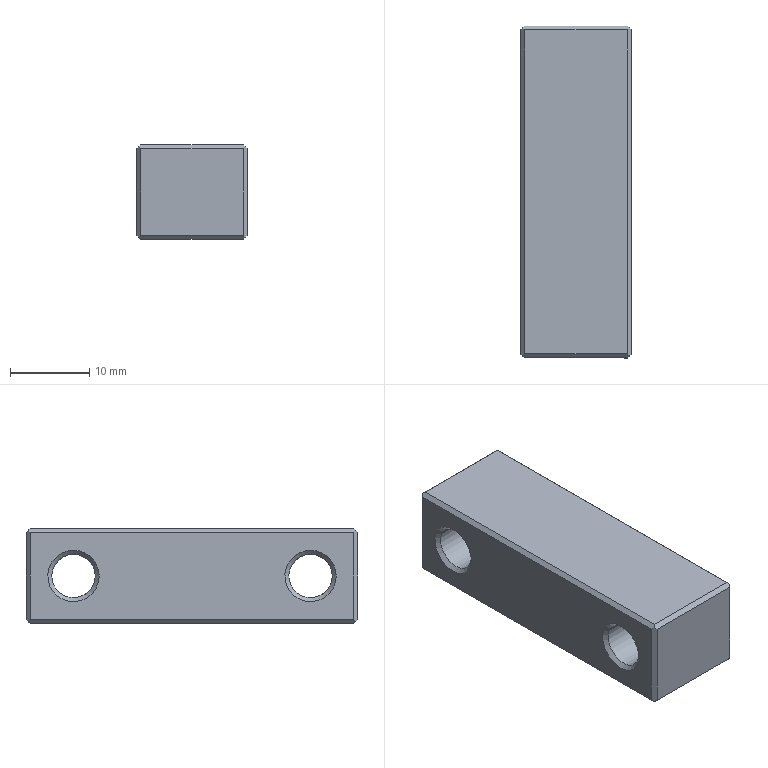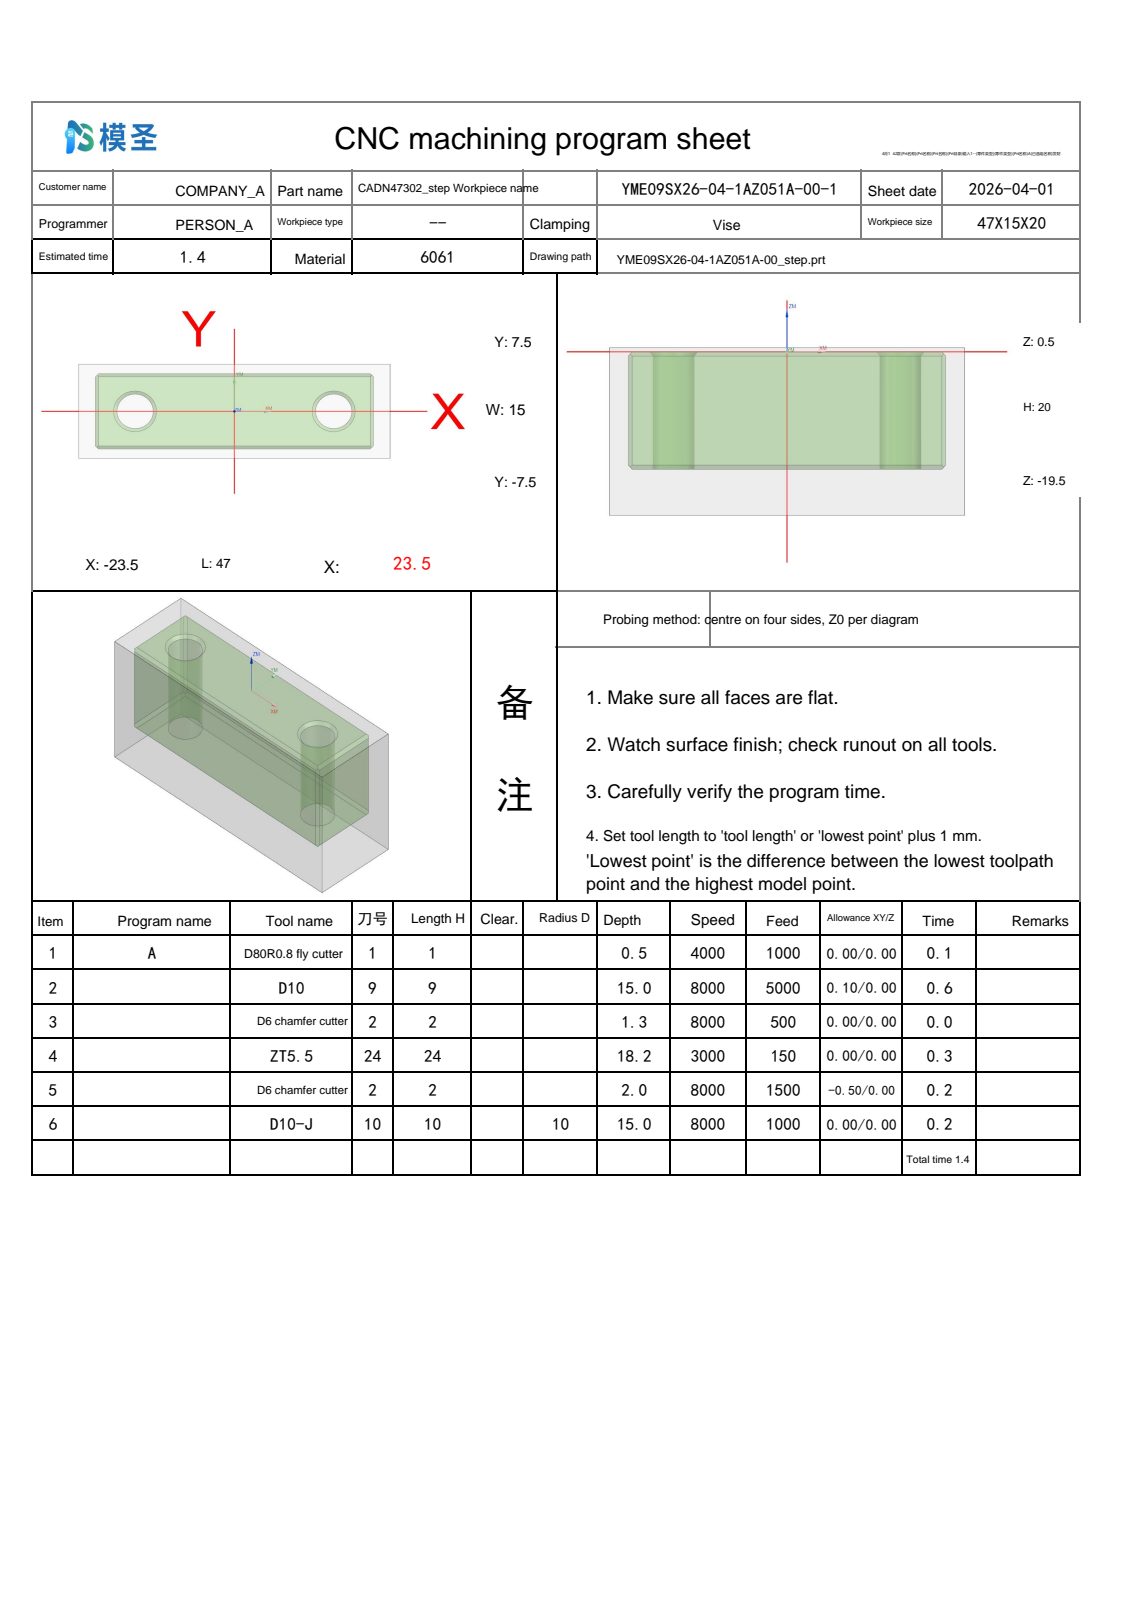NC program | NX | posted by the shop | part box 14 x 42 x 12 mm
Whole program:
%
O0001
(Machine time: 2.49 MIN)
(===Total Tool:5===)
(T1=D80R0.8 fly cutter D=80.  R=0.8  D-  H01 Z=0.    )
(T9=D10     D=10.  R=0.   D-  H09 Z=-14.5 )
(T2=D6 chamfer cutter   D=6.   R=0.   D-  H02 Z=-1.5  )
(T24=ZT5.5  D=5.5  DR_a=118 D-  H24 Z=-17.65)
(T10=D10-J  D=10.  R=0.   D10 H10 Z=-14.5 )
G80 G90 G17 G49 G40
G91 G28 Z0
M01
N1 T01 M06
(D80R0.8 fly cutter  D=80. R=0.8 H=01 ce=0.00 di=0.00)
G00 G90 G54 X-66. Y0.0 M03 S4000
G43 H01 Z20.
M08
Z2.
G01 Z0.0 F1000.
X-61.
X61.
X66.
Z2.
G00 Z20.
G91 G28 Z0.0
M05
M09
G91 G28 Z0.0
M01
N2 T09 M06
(D10  D=10. R=0. H=09 ce=0.10 di=0.00)
G00 G90 G54 X0.0 Y11.1 M03 S8000
G43 H09 Z20.
M08
Z.5
G01 X20.5 Z.383 F5000.
G02 X24.106 Y9.606 Z.361 I0.0 J-5.1
G01 X24.606 Y9.106 Z.357
G02 X26.1 Y5.5 Z.334 I-3.606 J-3.606
G01 Y-5.5 Z.271
G02 X24.606 Y-9.106 Z.249 I-5.1 J0.0
G01 X24.106 Y-9.606 Z.245
G02 X20.5 Y-11.1 Z.222 I-3.606 J3.606
G01 X-20.5 Z-.011
G02 X-24.106 Y-9.606 Z-.034 I0.0 J5.1
G01 X-24.606 Y-9.106 Z-.038
G02 X-26.1 Y-5.5 Z-.061 I3.606 J3.606
G01 Y5.5 Z-.123
G02 X-24.606 Y9.106 Z-.146 I5.1 J0.0
G01 X-24.106 Y9.606 Z-.15
G02 X-20.5 Y11.1 Z-.173 I3.606 J-3.606
G01 X20.5 Z-.406
G02 X24.106 Y9.606 Z-.429 I0.0 J-5.1
G01 X24.606 Y9.106 Z-.433
G02 X26.1 Y5.5 Z-.456 I-3.606 J-3.606
G01 Y-5.5 Z-.518
G02 X24.606 Y-9.106 Z-.541 I-5.1 J0.0
G01 X24.106 Y-9.606 Z-.545
G02 X20.5 Y-11.1 Z-.568 I-3.606 J3.606
G01 X-20.5 Z-.801
G02 X-24.106 Y-9.606 Z-.824 I0.0 J5.1
G01 X-24.606 Y-9.106 Z-.828
G02 X-26.1 Y-5.5 Z-.85 I3.606 J3.606
G01 Y5.5 Z-.913
G02 X-24.606 Y9.106 Z-.936 I5.1 J0.0
G01 X-24.106 Y9.606 Z-.94
G02 X-20.5 Y11.1 Z-.962 I3.606 J-3.606
G01 X20.5 Z-1.195
G02 X24.106 Y9.606 Z-1.218 I0.0 J-5.1
G01 X24.606 Y9.106 Z-1.222
G02 X26.1 Y5.5 Z-1.245 I-3.606 J-3.606
G01 Y-5.5 Z-1.308
G02 X24.606 Y-9.106 Z-1.33 I-5.1 J0.0
G01 X24.106 Y-9.606 Z-1.334
G02 X20.5 Y-11.1 Z-1.357 I-3.606 J3.606
G01 X-20.5 Z-1.59
G02 X-24.106 Y-9.606 Z-1.613 I0.0 J5.1
G01 X-24.606 Y-9.106 Z-1.617
G02 X-26.1 Y-5.5 Z-1.64 I3.606 J3.606
G01 Y5.5 Z-1.702
G02 X-24.606 Y9.106 Z-1.725 I5.1 J0.0
G01 X-24.106 Y9.606 Z-1.729
G02 X-20.5 Y11.1 Z-1.752 I3.606 J-3.606
G01 X20.5 Z-1.985
G02 X24.106 Y9.606 Z-2.008 I0.0 J-5.1
G01 X24.606 Y9.106 Z-2.012
G02 X26.1 Y5.5 Z-2.035 I-3.606 J-3.606
G01 Y-5.5 Z-2.097
G02 X24.606 Y-9.106 Z-2.12 I-5.1 J0.0
G01 X24.106 Y-9.606 Z-2.124
G02 X20.5 Y-11.1 Z-2.147 I-3.606 J3.606
G01 X-20.5 Z-2.38
G02 X-24.106 Y-9.606 Z-2.402 I0.0 J5.1
G01 X-24.606 Y-9.106 Z-2.406
G02 X-26.1 Y-5.5 Z-2.429 I3.606 J3.606
G01 Y5.5 Z-2.492
G02 X-24.606 Y9.106 Z-2.515 I5.1 J0.0
G01 X-24.106 Y9.606 Z-2.519
G02 X-20.5 Y11.1 Z-2.541 I3.606 J-3.606
G01 X20.5 Z-2.774
G02 X24.106 Y9.606 Z-2.797 I0.0 J-5.1
G01 X24.606 Y9.106 Z-2.801
G02 X26.1 Y5.5 Z-2.824 I-3.606 J-3.606
G01 Y-5.5 Z-2.887
G02 X24.606 Y-9.106 Z-2.909 I-5.1 J0.0
G01 X24.106 Y-9.606 Z-2.913
G02 X20.5 Y-11.1 Z-2.936 I-3.606 J3.606
G01 X-20.5 Z-3.169
G02 X-24.106 Y-9.606 Z-3.192 I0.0 J5.1
G01 X-24.606 Y-9.106 Z-3.196
G02 X-26.1 Y-5.5 Z-3.219 I3.606 J3.606
G01 Y5.5 Z-3.281
G02 X-24.606 Y9.106 Z-3.304 I5.1 J0.0
G01 X-24.106 Y9.606 Z-3.308
G02 X-20.5 Y11.1 Z-3.331 I3.606 J-3.606
G01 X20.5 Z-3.564
G02 X24.106 Y9.606 Z-3.587 I0.0 J-5.1
G01 X24.606 Y9.106 Z-3.591
G02 X26.1 Y5.5 Z-3.613 I-3.606 J-3.606
G01 Y-5.5 Z-3.676
G02 X24.606 Y-9.106 Z-3.699 I-5.1 J0.0
G01 X24.106 Y-9.606 Z-3.703
G02 X20.5 Y-11.1 Z-3.726 I-3.606 J3.606
G01 X-20.5 Z-3.959
G02 X-24.106 Y-9.606 Z-3.981 I0.0 J5.1
G01 X-24.606 Y-9.106 Z-3.985
G02 X-26.1 Y-5.5 Z-4.008 I3.606 J3.606
G01 Y5.5 Z-4.071
G02 X-24.606 Y9.106 Z-4.094 I5.1 J0.0
G01 X-24.106 Y9.606 Z-4.098
G02 X-20.5 Y11.1 Z-4.12 I3.606 J-3.606
G01 X20.5 Z-4.353
G02 X24.106 Y9.606 Z-4.376 I0.0 J-5.1
G01 X24.606 Y9.106 Z-4.38
G02 X26.1 Y5.5 Z-4.403 I-3.606 J-3.606
G01 Y-5.5 Z-4.465
G02 X24.606 Y-9.106 Z-4.488 I-5.1 J0.0
G01 X24.106 Y-9.606 Z-4.492
G02 X20.5 Y-11.1 Z-4.515 I-3.606 J3.606
G01 X-20.5 Z-4.748
G02 X-24.106 Y-9.606 Z-4.771 I0.0 J5.1
G01 X-24.606 Y-9.106 Z-4.775
G02 X-26.1 Y-5.5 Z-4.798 I3.606 J3.606
G01 Y5.5 Z-4.86
G02 X-24.606 Y9.106 Z-4.883 I5.1 J0.0
G01 X-24.106 Y9.606 Z-4.887
G02 X-20.5 Y11.1 Z-4.91 I3.606 J-3.606
G01 X20.5 Z-5.143
G02 X24.106 Y9.606 Z-5.166 I0.0 J-5.1
G01 X24.606 Y9.106 Z-5.17
G02 X26.1 Y5.5 Z-5.192 I-3.606 J-3.606
G01 Y-5.5 Z-5.255
G02 X24.606 Y-9.106 Z-5.278 I-5.1 J0.0
G01 X24.106 Y-9.606 Z-5.282
G02 X20.5 Y-11.1 Z-5.305 I-3.606 J3.606
G01 X-20.5 Z-5.538
G02 X-24.106 Y-9.606 Z-5.56 I0.0 J5.1
G01 X-24.606 Y-9.106 Z-5.564
G02 X-26.1 Y-5.5 Z-5.587 I3.606 J3.606
G01 Y5.5 Z-5.65
G02 X-24.606 Y9.106 Z-5.672 I5.1 J0.0
G01 X-24.106 Y9.606 Z-5.676
G02 X-20.5 Y11.1 Z-5.699 I3.606 J-3.606
G01 X20.5 Z-5.932
G02 X24.106 Y9.606 Z-5.955 I0.0 J-5.1
G01 X24.606 Y9.106 Z-5.959
G02 X26.1 Y5.5 Z-5.982 I-3.606 J-3.606
G01 Y-5.5 Z-6.044
G02 X24.606 Y-9.106 Z-6.067 I-5.1 J0.0
G01 X24.106 Y-9.606 Z-6.071
G02 X20.5 Y-11.1 Z-6.094 I-3.606 J3.606
G01 X-20.5 Z-6.327
G02 X-24.106 Y-9.606 Z-6.35 I0.0 J5.1
G01 X-24.606 Y-9.106 Z-6.354
G02 X-26.1 Y-5.5 Z-6.377 I3.606 J3.606
G01 Y5.5 Z-6.439
G02 X-24.606 Y9.106 Z-6.462 I5.1 J0.0
G01 X-24.106 Y9.606 Z-6.466
G02 X-20.5 Y11.1 Z-6.489 I3.606 J-3.606
G01 X20.5 Z-6.722
G02 X24.106 Y9.606 Z-6.745 I0.0 J-5.1
G01 X24.606 Y9.106 Z-6.749
G02 X26.1 Y5.5 Z-6.771 I-3.606 J-3.606
G01 Y-5.5 Z-6.834
G02 X24.606 Y-9.106 Z-6.857 I-5.1 J0.0
G01 X24.106 Y-9.606 Z-6.861
G02 X20.5 Y-11.1 Z-6.883 I-3.606 J3.606
G01 X-20.5 Z-7.117
G02 X-24.106 Y-9.606 Z-7.139 I0.0 J5.1
G01 X-24.606 Y-9.106 Z-7.143
G02 X-26.1 Y-5.5 Z-7.166 I3.606 J3.606
G01 Y5.5 Z-7.229
G02 X-24.606 Y9.106 Z-7.251 I5.1 J0.0
G01 X-24.106 Y9.606 Z-7.255
G02 X-20.5 Y11.1 Z-7.278 I3.606 J-3.606
G01 X20.5 Z-7.511
G02 X24.106 Y9.606 Z-7.534 I0.0 J-5.1
G01 X24.606 Y9.106 Z-7.538
G02 X26.1 Y5.5 Z-7.561 I-3.606 J-3.606
G01 Y-5.5 Z-7.623
G02 X24.606 Y-9.106 Z-7.646 I-5.1 J0.0
G01 X24.106 Y-9.606 Z-7.65
G02 X20.5 Y-11.1 Z-7.673 I-3.606 J3.606
G01 X-20.5 Z-7.906
G02 X-24.106 Y-9.606 Z-7.929 I0.0 J5.1
G01 X-24.606 Y-9.106 Z-7.933
G02 X-26.1 Y-5.5 Z-7.956 I3.606 J3.606
G01 Y5.5 Z-8.018
G02 X-24.606 Y9.106 Z-8.041 I5.1 J0.0
G01 X-24.106 Y9.606 Z-8.045
G02 X-20.5 Y11.1 Z-8.068 I3.606 J-3.606
G01 X20.5 Z-8.301
G02 X24.106 Y9.606 Z-8.324 I0.0 J-5.1
G01 X24.606 Y9.106 Z-8.328
G02 X26.1 Y5.5 Z-8.35 I-3.606 J-3.606
G01 Y-5.5 Z-8.413
G02 X24.606 Y-9.106 Z-8.436 I-5.1 J0.0
G01 X24.106 Y-9.606 Z-8.44
G02 X20.5 Y-11.1 Z-8.462 I-3.606 J3.606
G01 X-20.5 Z-8.695
G02 X-24.106 Y-9.606 Z-8.718 I0.0 J5.1
G01 X-24.606 Y-9.106 Z-8.722
G02 X-26.1 Y-5.5 Z-8.745 I3.606 J3.606
G01 Y5.5 Z-8.808
G02 X-24.606 Y9.106 Z-8.83 I5.1 J0.0
G01 X-24.106 Y9.606 Z-8.834
G02 X-20.5 Y11.1 Z-8.857 I3.606 J-3.606
G01 X20.5 Z-9.09
G02 X24.106 Y9.606 Z-9.113 I0.0 J-5.1
G01 X24.606 Y9.106 Z-9.117
G02 X26.1 Y5.5 Z-9.14 I-3.606 J-3.606
G01 Y-5.5 Z-9.202
G02 X24.606 Y-9.106 Z-9.225 I-5.1 J0.0
G01 X24.106 Y-9.606 Z-9.229
G02 X20.5 Y-11.1 Z-9.252 I-3.606 J3.606
G01 X-20.5 Z-9.485
G02 X-24.106 Y-9.606 Z-9.508 I0.0 J5.1
G01 X-24.606 Y-9.106 Z-9.512
G02 X-26.1 Y-5.5 Z-9.535 I3.606 J3.606
G01 Y5.5 Z-9.597
G02 X-24.606 Y9.106 Z-9.62 I5.1 J0.0
G01 X-24.106 Y9.606 Z-9.624
G02 X-20.5 Y11.1 Z-9.647 I3.606 J-3.606
G01 X20.5 Z-9.88
G02 X24.106 Y9.606 Z-9.902 I0.0 J-5.1
G01 X24.606 Y9.106 Z-9.906
G02 X26.1 Y5.5 Z-9.929 I-3.606 J-3.606
G01 Y-5.5 Z-9.992
G02 X24.606 Y-9.106 Z-10.015 I-5.1 J0.0
G01 X24.106 Y-9.606 Z-10.019
G02 X20.5 Y-11.1 Z-10.041 I-3.606 J3.606
G01 X-20.5 Z-10.274
G02 X-24.106 Y-9.606 Z-10.297 I0.0 J5.1
G01 X-24.606 Y-9.106 Z-10.301
G02 X-26.1 Y-5.5 Z-10.324 I3.606 J3.606
G01 Y5.5 Z-10.387
G02 X-24.606 Y9.106 Z-10.409 I5.1 J0.0
G01 X-24.106 Y9.606 Z-10.413
G02 X-20.5 Y11.1 Z-10.436 I3.606 J-3.606
G01 X20.5 Z-10.669
G02 X24.106 Y9.606 Z-10.692 I0.0 J-5.1
G01 X24.606 Y9.106 Z-10.696
G02 X26.1 Y5.5 Z-10.719 I-3.606 J-3.606
G01 Y-5.5 Z-10.781
G02 X24.606 Y-9.106 Z-10.804 I-5.1 J0.0
G01 X24.106 Y-9.606 Z-10.808
G02 X20.5 Y-11.1 Z-10.831 I-3.606 J3.606
G01 X-20.5 Z-11.064
G02 X-24.106 Y-9.606 Z-11.087 I0.0 J5.1
G01 X-24.606 Y-9.106 Z-11.091
G02 X-26.1 Y-5.5 Z-11.113 I3.606 J3.606
G01 Y5.5 Z-11.176
G02 X-24.606 Y9.106 Z-11.199 I5.1 J0.0
G01 X-24.106 Y9.606 Z-11.203
G02 X-20.5 Y11.1 Z-11.226 I3.606 J-3.606
G01 X20.5 Z-11.459
G02 X24.106 Y9.606 Z-11.481 I0.0 J-5.1
G01 X24.606 Y9.106 Z-11.485
G02 X26.1 Y5.5 Z-11.508 I-3.606 J-3.606
G01 Y-5.5 Z-11.571
G02 X24.606 Y-9.106 Z-11.594 I-5.1 J0.0
G01 X24.106 Y-9.606 Z-11.598
G02 X20.5 Y-11.1 Z-11.62 I-3.606 J3.606
G01 X-20.5 Z-11.853
G02 X-24.106 Y-9.606 Z-11.876 I0.0 J5.1
G01 X-24.606 Y-9.106 Z-11.88
G02 X-26.1 Y-5.5 Z-11.903 I3.606 J3.606
G01 Y5.5 Z-11.965
G02 X-24.606 Y9.106 Z-11.988 I5.1 J0.0
G01 X-24.106 Y9.606 Z-11.992
G02 X-20.5 Y11.1 Z-12.015 I3.606 J-3.606
G01 X20.5 Z-12.248
G02 X24.106 Y9.606 Z-12.271 I0.0 J-5.1
G01 X24.606 Y9.106 Z-12.275
G02 X26.1 Y5.5 Z-12.298 I-3.606 J-3.606
G01 Y-5.5 Z-12.36
G02 X24.606 Y-9.106 Z-12.383 I-5.1 J0.0
G01 X24.106 Y-9.606 Z-12.387
G02 X20.5 Y-11.1 Z-12.41 I-3.606 J3.606
G01 X-20.5 Z-12.643
G02 X-24.106 Y-9.606 Z-12.666 I0.0 J5.1
G01 X-24.606 Y-9.106 Z-12.67
G02 X-26.1 Y-5.5 Z-12.692 I3.606 J3.606
G01 Y5.5 Z-12.755
G02 X-24.606 Y9.106 Z-12.778 I5.1 J0.0
G01 X-24.106 Y9.606 Z-12.782
G02 X-20.5 Y11.1 Z-12.805 I3.606 J-3.606
G01 X20.5 Z-13.038
G02 X24.106 Y9.606 Z-13.06 I0.0 J-5.1
G01 X24.606 Y9.106 Z-13.064
G02 X26.1 Y5.5 Z-13.087 I-3.606 J-3.606
G01 Y-5.5 Z-13.15
G02 X24.606 Y-9.106 Z-13.172 I-5.1 J0.0
G01 X24.106 Y-9.606 Z-13.176
G02 X20.5 Y-11.1 Z-13.199 I-3.606 J3.606
G01 X-20.5 Z-13.432
G02 X-24.106 Y-9.606 Z-13.455 I0.0 J5.1
G01 X-24.606 Y-9.106 Z-13.459
G02 X-26.1 Y-5.5 Z-13.482 I3.606 J3.606
G01 Y5.5 Z-13.544
G02 X-24.606 Y9.106 Z-13.567 I5.1 J0.0
G01 X-24.106 Y9.606 Z-13.571
G02 X-20.5 Y11.1 Z-13.594 I3.606 J-3.606
G01 X20.5 Z-13.827
G02 X24.106 Y9.606 Z-13.85 I0.0 J-5.1
G01 X24.606 Y9.106 Z-13.854
G02 X26.1 Y5.5 Z-13.877 I-3.606 J-3.606
G01 Y-5.5 Z-13.939
G02 X24.606 Y-9.106 Z-13.962 I-5.1 J0.0
G01 X24.106 Y-9.606 Z-13.966
G02 X20.5 Y-11.1 Z-13.989 I-3.606 J3.606
G01 X-20.5 Z-14.222
G02 X-24.106 Y-9.606 Z-14.245 I0.0 J5.1
G01 X-24.606 Y-9.106 Z-14.249
G02 X-26.1 Y-5.5 Z-14.271 I3.606 J3.606
G01 Y5.5 Z-14.334
G02 X-24.606 Y9.106 Z-14.357 I5.1 J0.0
G01 X-24.106 Y9.606 Z-14.361
G02 X-20.5 Y11.1 Z-14.383 I3.606 J-3.606
G01 X0.0 Z-14.5
X20.5
G02 X24.106 Y9.606 I0.0 J-5.1
G01 X24.606 Y9.106
G02 X26.1 Y5.5 I-3.606 J-3.606
G01 Y-5.5
G02 X24.606 Y-9.106 I-5.1 J0.0
G01 X24.106 Y-9.606
G02 X20.5 Y-11.1 I-3.606 J3.606
G01 X-20.5
G02 X-24.106 Y-9.606 I0.0 J5.1
G01 X-24.606 Y-9.106
G02 X-26.1 Y-5.5 I3.606 J3.606
G01 Y5.5
G02 X-24.606 Y9.106 I5.1 J0.0
G01 X-24.106 Y9.606
G02 X-20.5 Y11.1 I3.606 J-3.606
G01 X0.0
X.5
Z-13.5
G00 Z20.
G91 G28 Z0.0
M05
M09
G91 G28 Z0.0
M01
N3 T02 M06
(D6 chamfer cutter  D=6. R=0. H=02 ce=0.00 di=0.00)
G00 G90 G54 X15. Y0.0 M03 S8000
G43 H02 Z20.
M08
G98 G81 X15. Y0.0 Z-.8 R1. F500.
X-15.
G80
G00 Z20.
G91 G28 Z0.0
M05
M09
G91 G28 Z0.0
M01
N4 T24 M06
(ZT5.5 D=5.5 DR_a=118 H=24)
G00 G90 G54 X15. Y0.0 M03 S3000
G43 H24 Z20.
M08
G98 G83 X15. Y0.0 Z-17.652 R1. F150. Q3.
X-15.
G80
G00 Z20.
G91 G28 Z0.0
M05
M09
G91 G28 Z0.0
M01
N5 T02 M06
(D6 chamfer cutter  D=6. R=0. H=02 ce=-0.50 di=0.00)
G00 G90 G54 X15.74 Y.123 M03 S8000
G43 H02 Z20.
M08
Z-1.
G01 Z-1.5 F500.
X16.5 Y.25
G03 X15. Y1.75 I-1.5 J0.0
X13.25 Y0.0 I0.0 J-1.75
X15. Y-1.75 I1.75 J0.0
X16.75 Y0.0 I0.0 J1.75
X15. Y1.75 I-1.75 J0.0
X13.5 Y.25 I0.0 J-1.5
G01 X14.26 Y.123
Z-1.
G00 Z20.
X-14.26
Z-1.
G01 Z-1.5
X-13.5 Y.25
G03 X-15. Y1.75 I-1.5 J0.0
X-16.75 Y0.0 I0.0 J-1.75
X-15. Y-1.75 I1.75 J0.0
X-13.25 Y0.0 I0.0 J1.75
X-15. Y1.75 I-1.75 J0.0
X-16.5 Y.25 I0.0 J-1.5
G01 X-15.74 Y.123
Z-1.
G00 Z20.
G00 G90 X22.517 Y-7.021 M03 S6500
Z20.
Z.3
G01 Z-1.2 F1500.
G03 X21.7 Y-6.7 I-.817 J-.879
G01 X-21.7
Y6.7
X21.7
Y-6.7
X21.3
G03 X20.1 Y-7.9 I0.0 J-1.2
G01 Z.3
G00 Z20.
G91 G28 Z0.0
M05
M09
G91 G28 Z0.0
M01
N6 T10 M06
(D10-J  D=10. R=0. H=10 ce=0.00 di=0.00)
G00 G90 G54 X21.513 Y-12.116 M03 S8000
G43 H10 Z20.
M08
Z-14.
G01 Z-14.5 F1000.
G41 D10
X21.497 Y-11.917
G03 X20.5 Y-11. I-.997 J-.083
G01 X-20.5
G02 X-24.036 Y-9.536 I0.0 J5.
G01 X-24.536 Y-9.036
G02 X-26. Y-5.5 I3.536 J3.536
G01 Y5.5
G02 X-24.536 Y9.036 I5. J0.0
G01 X-24.036 Y9.536
G02 X-20.5 Y11. I3.536 J-3.536
G01 X20.5
G02 X24.036 Y9.536 I0.0 J-5.
G01 X24.536 Y9.036
G02 X26. Y5.5 I-3.536 J-3.536
G01 Y-5.5
G02 X24.536 Y-9.036 I-5. J0.0
G01 X24.036 Y-9.536
G02 X20.5 Y-11. I-3.536 J3.536
G01 X20.
G03 X19. Y-12. I0.0 J-1.
G01 G40 Y-12.2
Z-14.
G00 Z20.
M05
M09
G91 G28 Z0.0
G91 G28 Y0.0
M30
%